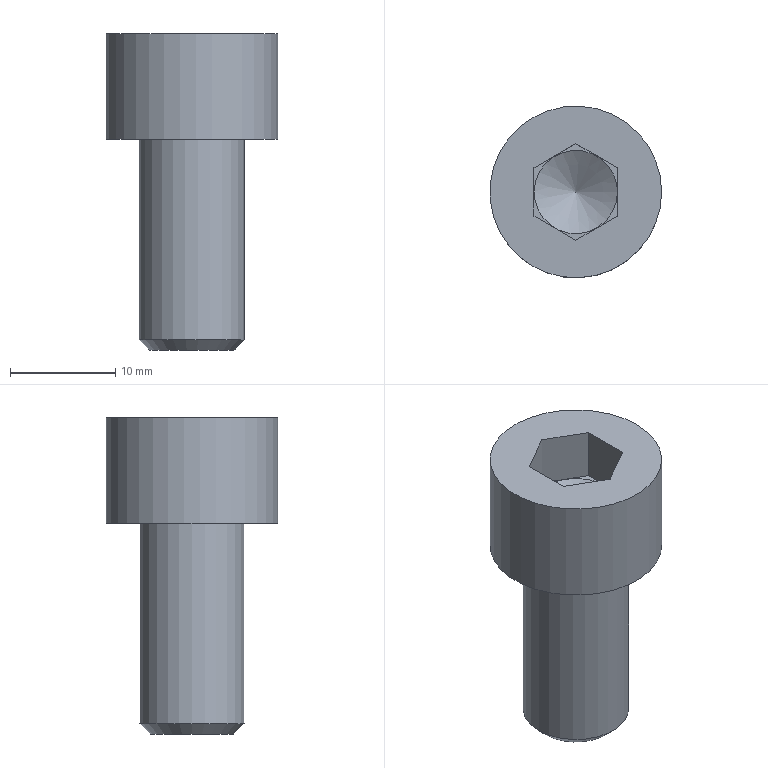Part | NX | features BOLT(M1020_GB70-85).1 2 | 1 solid | 14 faces | box 16.28 x 16.28 x 30 mm | volume 3328 mm3 | plane 10 | cone 2 | cylinder 2 | commonest cylinder face diameters 10 x1 16.28 x1
STEP:
#1=CARTESIAN_POINT('',(-841.86,640.,-95.));
#2=VERTEX_POINT('',#1);
#3=CARTESIAN_POINT('',(-850.,640.,-95.));
#4=DIRECTION('',(0.,0.,-1.));
#5=DIRECTION('',(1.,0.,0.));
#6=AXIS2_PLACEMENT_3D('',#3,#4,#5);
#7=CIRCLE('',#6,8.14);
#8=EDGE_CURVE('',#2,#2,#7,.T.);
#9=ORIENTED_EDGE('',*,*,#8,.T.);
#10=EDGE_LOOP('',(#9));
#11=FACE_BOUND('',#10,.T.);
#12=CARTESIAN_POINT('',(-845.,640.,-95.));
#13=VERTEX_POINT('',#12);
#14=CARTESIAN_POINT('',(-850.,640.,-95.));
#15=DIRECTION('',(0.,0.,1.));
#16=DIRECTION('',(1.,0.,0.));
#17=AXIS2_PLACEMENT_3D('',#14,#15,#16);
#18=CIRCLE('',#17,5.);
#19=EDGE_CURVE('',#13,#13,#18,.T.);
#20=ORIENTED_EDGE('',*,*,#19,.T.);
#21=EDGE_LOOP('',(#20));
#22=FACE_BOUND('',#21,.T.);
#23=CARTESIAN_POINT('',(-894.667,672.579,-95.));
#24=DIRECTION('',(0.,0.,1.));
#25=DIRECTION('',(1.,0.,0.));
#26=AXIS2_PLACEMENT_3D('',#23,#24,#25);
#27=PLANE('',#26);
#28=ADVANCED_FACE('',(#11,#22),#27,.F.);
#29=CARTESIAN_POINT('',(-853.95,640.,-90.01));
#30=VERTEX_POINT('',#29);
#31=CARTESIAN_POINT('',(-853.727,638.393,-90.));
#32=CARTESIAN_POINT('',(-854.053,639.948,-90.));
#33=CARTESIAN_POINT('',(-853.76,641.497,-90.));
#34=CARTESIAN_POINT('',(-852.924,642.806,-90.));
#35=CARTESIAN_POINT('',(-851.629,643.711,-90.));
#36=CARTESIAN_POINT('',(-850.085,644.052,-90.));
#37=CARTESIAN_POINT('',(-848.528,643.776,-90.));
#38=CARTESIAN_POINT('',(-847.195,642.925,-90.));
#39=CARTESIAN_POINT('',(-846.289,641.629,-90.));
#40=CARTESIAN_POINT('',(-845.948,640.085,-90.));
#41=CARTESIAN_POINT('',(-846.224,638.528,-90.));
#42=CARTESIAN_POINT('',(-847.075,637.195,-90.));
#43=CARTESIAN_POINT('',(-848.371,636.289,-90.));
#44=CARTESIAN_POINT('',(-849.915,635.948,-90.));
#45=CARTESIAN_POINT('',(-851.472,636.224,-90.));
#46=CARTESIAN_POINT('',(-852.805,637.075,-90.));
#47=CARTESIAN_POINT('',(-853.727,638.393,-90.));
#48=CARTESIAN_POINT('',(-854.053,639.948,-90.));
#49=CARTESIAN_POINT('',(-853.76,641.497,-90.));
#50=B_SPLINE_CURVE_WITH_KNOTS('',3,(#31,#32,#33,#34,#35,#36,#37,#38,#39,#40,#41,#42,#43,#44,#45,#46,#47,#48,#49),.UNSPECIFIED.,.T.,.F.,(1,1,1,1,1,1,1,1,1,1,1,1,1,1,1,1,1,1,1,1,1,1,1),(-0.1908,-0.1283,-0.06579,0.,0.05937,0.1217,0.1842,0.2467,0.3092,0.3717,0.4342,0.4967,0.5592,0.6217,0.6842,0.7467,0.8092,0.8717,0.9342,1.,1.059,1.122,1.184),.UNSPECIFIED.);
#51=EDGE_CURVE('',#30,#30,#50,.F.);
#52=ORIENTED_EDGE('',*,*,#51,.T.);
#53=EDGE_LOOP('',(#52));
#54=FACE_BOUND('',#53,.T.);
#55=CARTESIAN_POINT('',(-850.,640.,-92.291));
#56=VERTEX_POINT('',#55);
#57=VERTEX_LOOP('',#56);
#58=FACE_BOUND('',#57,.T.);
#59=CARTESIAN_POINT('',(-850.,640.,-92.291));
#60=DIRECTION('',(0.,0.,1.));
#61=DIRECTION('',(1.,0.,0.));
#62=AXIS2_PLACEMENT_3D('',#59,#60,#61);
#63=CONICAL_SURFACE('',#62,0.,1.047);
#64=ADVANCED_FACE('',(#54,#58),#63,.F.);
#65=CARTESIAN_POINT('',(-853.966,637.71,-90.));
#66=VERTEX_POINT('',#65);
#67=CARTESIAN_POINT('',(-853.966,642.29,-90.));
#68=VERTEX_POINT('',#67);
#69=CARTESIAN_POINT('',(-853.966,640.,-90.));
#70=DIRECTION('',(0.,1.,0.));
#71=VECTOR('',#70,1000.);
#72=LINE('',#69,#71);
#73=EDGE_CURVE('',#66,#68,#72,.T.);
#74=ORIENTED_EDGE('',*,*,#73,.T.);
#75=CARTESIAN_POINT('',(-853.966,642.29,-85.));
#76=VERTEX_POINT('',#75);
#77=CARTESIAN_POINT('',(-853.966,642.29,-87.5));
#78=DIRECTION('',(0.,0.,-1.));
#79=VECTOR('',#78,1000.);
#80=LINE('',#77,#79);
#81=EDGE_CURVE('',#76,#68,#80,.T.);
#82=ORIENTED_EDGE('',*,*,#81,.F.);
#83=CARTESIAN_POINT('',(-853.966,637.71,-85.));
#84=VERTEX_POINT('',#83);
#85=CARTESIAN_POINT('',(-853.966,640.,-85.));
#86=DIRECTION('',(0.,1.,0.));
#87=VECTOR('',#86,1000.);
#88=LINE('',#85,#87);
#89=EDGE_CURVE('',#84,#76,#88,.T.);
#90=ORIENTED_EDGE('',*,*,#89,.F.);
#91=CARTESIAN_POINT('',(-853.966,637.71,-87.5));
#92=DIRECTION('',(0.,0.,-1.));
#93=VECTOR('',#92,1000.);
#94=LINE('',#91,#93);
#95=EDGE_CURVE('',#84,#66,#94,.T.);
#96=ORIENTED_EDGE('',*,*,#95,.T.);
#97=EDGE_LOOP('',(#74,#82,#90,#96));
#98=FACE_BOUND('',#97,.T.);
#99=CARTESIAN_POINT('',(-853.966,637.71,-85.));
#100=DIRECTION('',(-1.,0.,0.));
#101=DIRECTION('',(0.,0.,1.));
#102=AXIS2_PLACEMENT_3D('',#99,#100,#101);
#103=PLANE('',#102);
#104=ADVANCED_FACE('',(#98),#103,.F.);
#105=CARTESIAN_POINT('',(-850.,644.58,-90.));
#106=VERTEX_POINT('',#105);
#107=CARTESIAN_POINT('',(-851.983,643.435,-90.));
#108=DIRECTION('',(0.866,0.5,0.));
#109=VECTOR('',#108,1000.);
#110=LINE('',#107,#109);
#111=EDGE_CURVE('',#68,#106,#110,.T.);
#112=ORIENTED_EDGE('',*,*,#111,.T.);
#113=CARTESIAN_POINT('',(-850.,644.58,-85.));
#114=VERTEX_POINT('',#113);
#115=CARTESIAN_POINT('',(-850.,644.58,-87.5));
#116=DIRECTION('',(0.,0.,-1.));
#117=VECTOR('',#116,1000.);
#118=LINE('',#115,#117);
#119=EDGE_CURVE('',#114,#106,#118,.T.);
#120=ORIENTED_EDGE('',*,*,#119,.F.);
#121=CARTESIAN_POINT('',(-851.983,643.435,-85.));
#122=DIRECTION('',(0.866,0.5,0.));
#123=VECTOR('',#122,1000.);
#124=LINE('',#121,#123);
#125=EDGE_CURVE('',#76,#114,#124,.T.);
#126=ORIENTED_EDGE('',*,*,#125,.F.);
#127=ORIENTED_EDGE('',*,*,#81,.T.);
#128=EDGE_LOOP('',(#112,#120,#126,#127));
#129=FACE_BOUND('',#128,.T.);
#130=CARTESIAN_POINT('',(-853.966,642.29,-85.));
#131=DIRECTION('',(-0.5,0.866,0.));
#132=DIRECTION('',(-0.866,-0.5,0.));
#133=AXIS2_PLACEMENT_3D('',#130,#131,#132);
#134=PLANE('',#133);
#135=ADVANCED_FACE('',(#129),#134,.F.);
#136=CARTESIAN_POINT('',(-846.034,642.29,-90.));
#137=VERTEX_POINT('',#136);
#138=CARTESIAN_POINT('',(-848.017,643.435,-90.));
#139=DIRECTION('',(0.866,-0.5,0.));
#140=VECTOR('',#139,1000.);
#141=LINE('',#138,#140);
#142=EDGE_CURVE('',#106,#137,#141,.T.);
#143=ORIENTED_EDGE('',*,*,#142,.T.);
#144=CARTESIAN_POINT('',(-846.034,642.29,-85.));
#145=VERTEX_POINT('',#144);
#146=CARTESIAN_POINT('',(-846.034,642.29,-87.5));
#147=DIRECTION('',(0.,0.,-1.));
#148=VECTOR('',#147,1000.);
#149=LINE('',#146,#148);
#150=EDGE_CURVE('',#145,#137,#149,.T.);
#151=ORIENTED_EDGE('',*,*,#150,.F.);
#152=CARTESIAN_POINT('',(-848.017,643.435,-85.));
#153=DIRECTION('',(0.866,-0.5,0.));
#154=VECTOR('',#153,1000.);
#155=LINE('',#152,#154);
#156=EDGE_CURVE('',#114,#145,#155,.T.);
#157=ORIENTED_EDGE('',*,*,#156,.F.);
#158=ORIENTED_EDGE('',*,*,#119,.T.);
#159=EDGE_LOOP('',(#143,#151,#157,#158));
#160=FACE_BOUND('',#159,.T.);
#161=CARTESIAN_POINT('',(-850.,644.58,-85.));
#162=DIRECTION('',(0.5,0.866,0.));
#163=DIRECTION('',(-0.866,0.5,0.));
#164=AXIS2_PLACEMENT_3D('',#161,#162,#163);
#165=PLANE('',#164);
#166=ADVANCED_FACE('',(#160),#165,.F.);
#167=CARTESIAN_POINT('',(-846.034,637.71,-90.));
#168=VERTEX_POINT('',#167);
#169=CARTESIAN_POINT('',(-846.034,640.,-90.));
#170=DIRECTION('',(0.,-1.,0.));
#171=VECTOR('',#170,1000.);
#172=LINE('',#169,#171);
#173=EDGE_CURVE('',#137,#168,#172,.T.);
#174=ORIENTED_EDGE('',*,*,#173,.T.);
#175=CARTESIAN_POINT('',(-846.034,637.71,-85.));
#176=VERTEX_POINT('',#175);
#177=CARTESIAN_POINT('',(-846.034,637.71,-87.5));
#178=DIRECTION('',(0.,0.,-1.));
#179=VECTOR('',#178,1000.);
#180=LINE('',#177,#179);
#181=EDGE_CURVE('',#176,#168,#180,.T.);
#182=ORIENTED_EDGE('',*,*,#181,.F.);
#183=CARTESIAN_POINT('',(-846.034,640.,-85.));
#184=DIRECTION('',(0.,-1.,0.));
#185=VECTOR('',#184,1000.);
#186=LINE('',#183,#185);
#187=EDGE_CURVE('',#145,#176,#186,.T.);
#188=ORIENTED_EDGE('',*,*,#187,.F.);
#189=ORIENTED_EDGE('',*,*,#150,.T.);
#190=EDGE_LOOP('',(#174,#182,#188,#189));
#191=FACE_BOUND('',#190,.T.);
#192=CARTESIAN_POINT('',(-846.034,642.29,-85.));
#193=DIRECTION('',(1.,0.,0.));
#194=DIRECTION('',(0.,0.,-1.));
#195=AXIS2_PLACEMENT_3D('',#192,#193,#194);
#196=PLANE('',#195);
#197=ADVANCED_FACE('',(#191),#196,.F.);
#198=CARTESIAN_POINT('',(-850.,635.42,-90.));
#199=VERTEX_POINT('',#198);
#200=CARTESIAN_POINT('',(-848.017,636.565,-90.));
#201=DIRECTION('',(-0.866,-0.5,0.));
#202=VECTOR('',#201,1000.);
#203=LINE('',#200,#202);
#204=EDGE_CURVE('',#168,#199,#203,.T.);
#205=ORIENTED_EDGE('',*,*,#204,.T.);
#206=CARTESIAN_POINT('',(-850.,635.42,-85.));
#207=VERTEX_POINT('',#206);
#208=CARTESIAN_POINT('',(-850.,635.42,-87.5));
#209=DIRECTION('',(0.,0.,-1.));
#210=VECTOR('',#209,1000.);
#211=LINE('',#208,#210);
#212=EDGE_CURVE('',#207,#199,#211,.T.);
#213=ORIENTED_EDGE('',*,*,#212,.F.);
#214=CARTESIAN_POINT('',(-848.017,636.565,-85.));
#215=DIRECTION('',(-0.866,-0.5,0.));
#216=VECTOR('',#215,1000.);
#217=LINE('',#214,#216);
#218=EDGE_CURVE('',#176,#207,#217,.T.);
#219=ORIENTED_EDGE('',*,*,#218,.F.);
#220=ORIENTED_EDGE('',*,*,#181,.T.);
#221=EDGE_LOOP('',(#205,#213,#219,#220));
#222=FACE_BOUND('',#221,.T.);
#223=CARTESIAN_POINT('',(-846.034,637.71,-85.));
#224=DIRECTION('',(0.5,-0.866,0.));
#225=DIRECTION('',(0.866,0.5,0.));
#226=AXIS2_PLACEMENT_3D('',#223,#224,#225);
#227=PLANE('',#226);
#228=ADVANCED_FACE('',(#222),#227,.F.);
#229=CARTESIAN_POINT('',(-851.983,636.565,-90.));
#230=DIRECTION('',(-0.866,0.5,0.));
#231=VECTOR('',#230,1000.);
#232=LINE('',#229,#231);
#233=EDGE_CURVE('',#199,#66,#232,.T.);
#234=ORIENTED_EDGE('',*,*,#233,.T.);
#235=ORIENTED_EDGE('',*,*,#95,.F.);
#236=CARTESIAN_POINT('',(-851.983,636.565,-85.));
#237=DIRECTION('',(-0.866,0.5,0.));
#238=VECTOR('',#237,1000.);
#239=LINE('',#236,#238);
#240=EDGE_CURVE('',#207,#84,#239,.T.);
#241=ORIENTED_EDGE('',*,*,#240,.F.);
#242=ORIENTED_EDGE('',*,*,#212,.T.);
#243=EDGE_LOOP('',(#234,#235,#241,#242));
#244=FACE_BOUND('',#243,.T.);
#245=CARTESIAN_POINT('',(-850.,635.42,-85.));
#246=DIRECTION('',(-0.5,-0.866,0.));
#247=DIRECTION('',(0.866,-0.5,0.));
#248=AXIS2_PLACEMENT_3D('',#245,#246,#247);
#249=PLANE('',#248);
#250=ADVANCED_FACE('',(#244),#249,.F.);
#251=CARTESIAN_POINT('',(-841.86,640.,-85.));
#252=VERTEX_POINT('',#251);
#253=CARTESIAN_POINT('',(-850.,640.,-85.));
#254=DIRECTION('',(0.,0.,-1.));
#255=DIRECTION('',(1.,0.,0.));
#256=AXIS2_PLACEMENT_3D('',#253,#254,#255);
#257=CIRCLE('',#256,8.14);
#258=EDGE_CURVE('',#252,#252,#257,.T.);
#259=ORIENTED_EDGE('',*,*,#258,.F.);
#260=EDGE_LOOP('',(#259));
#261=FACE_BOUND('',#260,.T.);
#262=ORIENTED_EDGE('',*,*,#240,.T.);
#263=ORIENTED_EDGE('',*,*,#89,.T.);
#264=ORIENTED_EDGE('',*,*,#125,.T.);
#265=ORIENTED_EDGE('',*,*,#156,.T.);
#266=ORIENTED_EDGE('',*,*,#187,.T.);
#267=ORIENTED_EDGE('',*,*,#218,.T.);
#268=EDGE_LOOP('',(#262,#263,#264,#265,#266,#267));
#269=FACE_BOUND('',#268,.T.);
#270=CARTESIAN_POINT('',(-894.667,672.579,-85.));
#271=DIRECTION('',(0.,0.,1.));
#272=DIRECTION('',(1.,0.,0.));
#273=AXIS2_PLACEMENT_3D('',#270,#271,#272);
#274=PLANE('',#273);
#275=ADVANCED_FACE('',(#261,#269),#274,.T.);
#276=ORIENTED_EDGE('',*,*,#258,.T.);
#277=EDGE_LOOP('',(#276));
#278=FACE_BOUND('',#277,.T.);
#279=ORIENTED_EDGE('',*,*,#8,.F.);
#280=EDGE_LOOP('',(#279));
#281=FACE_BOUND('',#280,.T.);
#282=CARTESIAN_POINT('',(-850.,640.,-90.));
#283=DIRECTION('',(0.,0.,-1.));
#284=DIRECTION('',(-1.,0.,0.));
#285=AXIS2_PLACEMENT_3D('',#282,#283,#284);
#286=CYLINDRICAL_SURFACE('',#285,8.14);
#287=ADVANCED_FACE('',(#278,#281),#286,.T.);
#288=ORIENTED_EDGE('',*,*,#233,.F.);
#289=ORIENTED_EDGE('',*,*,#204,.F.);
#290=ORIENTED_EDGE('',*,*,#173,.F.);
#291=ORIENTED_EDGE('',*,*,#142,.F.);
#292=ORIENTED_EDGE('',*,*,#111,.F.);
#293=ORIENTED_EDGE('',*,*,#73,.F.);
#294=EDGE_LOOP('',(#288,#289,#290,#291,#292,#293));
#295=FACE_BOUND('',#294,.T.);
#296=ORIENTED_EDGE('',*,*,#51,.F.);
#297=EDGE_LOOP('',(#296));
#298=FACE_BOUND('',#297,.T.);
#299=CARTESIAN_POINT('',(-894.667,672.579,-90.));
#300=DIRECTION('',(0.,0.,1.));
#301=DIRECTION('',(1.,0.,0.));
#302=AXIS2_PLACEMENT_3D('',#299,#300,#301);
#303=PLANE('',#302);
#304=ADVANCED_FACE('',(#295,#298),#303,.T.);
#305=CARTESIAN_POINT('',(-845.,640.,-114.));
#306=VERTEX_POINT('',#305);
#307=CARTESIAN_POINT('',(-850.,640.,-114.));
#308=DIRECTION('',(0.,0.,1.));
#309=DIRECTION('',(1.,0.,0.));
#310=AXIS2_PLACEMENT_3D('',#307,#308,#309);
#311=CIRCLE('',#310,5.);
#312=EDGE_CURVE('',#306,#306,#311,.T.);
#313=ORIENTED_EDGE('',*,*,#312,.T.);
#314=EDGE_LOOP('',(#313));
#315=FACE_BOUND('',#314,.T.);
#316=ORIENTED_EDGE('',*,*,#19,.F.);
#317=EDGE_LOOP('',(#316));
#318=FACE_BOUND('',#317,.T.);
#319=CARTESIAN_POINT('',(-850.,640.,-105.));
#320=DIRECTION('',(0.,0.,1.));
#321=DIRECTION('',(1.,0.,0.));
#322=AXIS2_PLACEMENT_3D('',#319,#320,#321);
#323=CYLINDRICAL_SURFACE('',#322,5.);
#324=ADVANCED_FACE('',(#315,#318),#323,.T.);
#325=CARTESIAN_POINT('',(-854.,640.,-115.));
#326=VERTEX_POINT('',#325);
#327=CARTESIAN_POINT('',(-850.,640.,-115.));
#328=DIRECTION('',(0.,0.,1.));
#329=DIRECTION('',(-1.,0.,0.));
#330=AXIS2_PLACEMENT_3D('',#327,#328,#329);
#331=CIRCLE('',#330,4.);
#332=EDGE_CURVE('',#326,#326,#331,.T.);
#333=ORIENTED_EDGE('',*,*,#332,.F.);
#334=EDGE_LOOP('',(#333));
#335=FACE_BOUND('',#334,.T.);
#336=CARTESIAN_POINT('',(-894.667,672.579,-115.));
#337=DIRECTION('',(0.,0.,-1.));
#338=DIRECTION('',(-1.,0.,0.));
#339=AXIS2_PLACEMENT_3D('',#336,#337,#338);
#340=PLANE('',#339);
#341=ADVANCED_FACE('',(#335),#340,.T.);
#342=ORIENTED_EDGE('',*,*,#332,.T.);
#343=EDGE_LOOP('',(#342));
#344=FACE_BOUND('',#343,.T.);
#345=ORIENTED_EDGE('',*,*,#312,.F.);
#346=EDGE_LOOP('',(#345));
#347=FACE_BOUND('',#346,.T.);
#348=CARTESIAN_POINT('',(-850.,640.,-119.));
#349=DIRECTION('',(0.,0.,1.));
#350=DIRECTION('',(1.,0.,0.));
#351=AXIS2_PLACEMENT_3D('',#348,#349,#350);
#352=CONICAL_SURFACE('',#351,0.,0.7854);
#353=ADVANCED_FACE('',(#344,#347),#352,.T.);
#354=CLOSED_SHELL('',(#28,#64,#104,#135,#166,#197,#228,#250,#275,#287,#304,#324,#341,#353));
#355=MANIFOLD_SOLID_BREP('',#354);
#356=(LENGTH_UNIT()NAMED_UNIT(*)SI_UNIT(.MILLI.,.METRE.));
#357=UNCERTAINTY_MEASURE_WITH_UNIT(LENGTH_MEASURE(0.0508),#356,'','');
#358=(NAMED_UNIT(*)PLANE_ANGLE_UNIT()SI_UNIT($,.RADIAN.));
#359=(NAMED_UNIT(*)SI_UNIT($,.STERADIAN.)SOLID_ANGLE_UNIT());
#360=(GEOMETRIC_REPRESENTATION_CONTEXT(3)GLOBAL_UNCERTAINTY_ASSIGNED_CONTEXT((#357))GLOBAL_UNIT_ASSIGNED_CONTEXT((#356,#358,#359))REPRESENTATION_CONTEXT('',''));
#361=ADVANCED_BREP_SHAPE_REPRESENTATION('',(#355),#360);